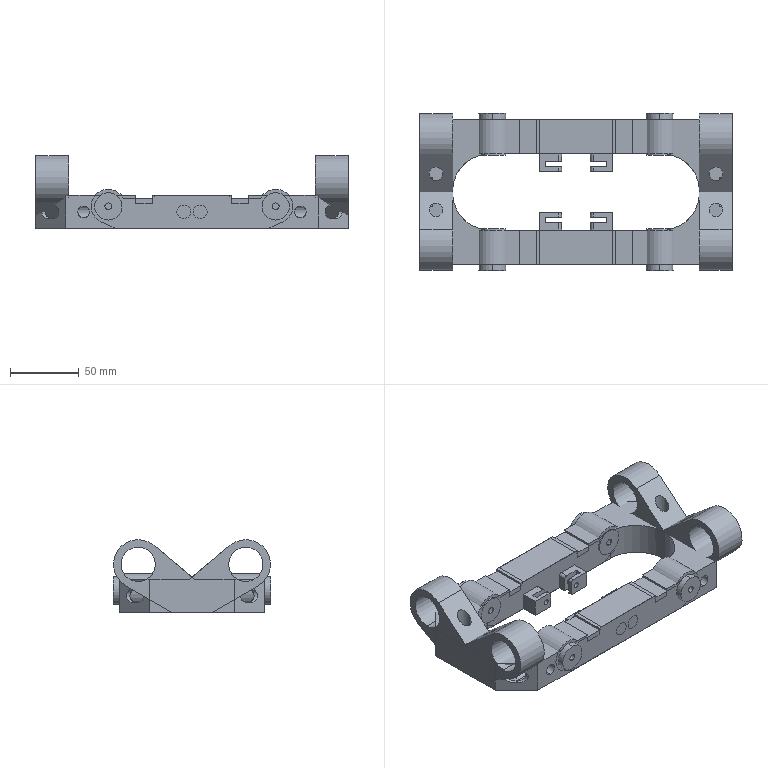NC program | Mastercam | posted with a generic post | part box 228 x 114.503 x 53 mm
Lines 1 to 872 of 11407:
%
:0001()
(MATERIAL - ALUMINUM MM - 2024)
(T12|12 FEM |H12|XY STOCK TO LEAVE - .25|Z STOCK TO LEAVE - .2)
(T7|6 CHM |H7)
(T3|10 BM/BNOS |H3)
(T4|4 BM/BNOS |H4)
N100 G21
N102 G0 G17 G40 G80 G90 G94 G98
N104 G0 G28 G91 Z0.
N106 G0 G28 X0. Y0.
(12 FEM |TOOL - 12|DIA. OFF. - 12|LEN. - 12|TOOL DIA. - 12.)
N108 T12 M6
N110 G0 G54 G90 X181.749 Y4.475 C0. B0. S6000 M3
N112 G43 H12 Z118.
N114 Z41.
N116 G1 Z38.275 F600.
N118 Y5.677 Z38.239 F6000.
N120 G3 X178.852 Y8.574 Z38.134 I-2.897
N122 G1 X177.889 Z38.121
N124 X166.677 Z37.774
N126 G3 X164.717 Y7.973 Z37.712 J-3.498
N128 X163.761 Y7.008 Z37.67 I1.96 J-2.897
N130 G2 X160.254 Y2.986 Z37.508 I-18.624 J12.704
N132 G3 X159.975 Y2.379 I.521 J-.607
N134 X160.775 Y1.578 I.8
N136 G1 X163.085
N138 X178.852
N140 G3 X181.749 Y4.475 J2.897
N142 G1 Y5.677
N144 G3 X178.852 Y8.574 I-2.897
N146 G1 X172.464
N148 X166.677
N150 G3 X163.761 Y7.008 J-3.498
N152 G2 X160.254 Y2.986 I-18.624 J12.704
N154 G3 X159.975 Y2.379 I.521 J-.607
N156 X160.775 Y1.578 I.8
N158 G1 X163.085
N160 G2 X164.255 Y.741 J-1.238
N162 G1 X165.626 Y-3.263
N164 G3 X166.797 Y-4.1 I1.171 J.401
N166 G1 X184.529
N168 G3 X187.427 Y-1.203 J2.897
N170 G1 Y11.354
N172 G3 X184.529 Y14.251 I-2.898
N174 G1 X172.464
N176 X164.58
N178 G3 X159.608 Y11.184 J-5.563
N180 G2 X155.054 Y6.215 I-12.896 J7.248
N182 G3 X153.144 Y2.669 I2.337 J-3.546
N184 X153.183 Y2.093 I4.247
N186 G1 X153.297 Y-1.203
N188 G3 X156.194 Y-4.1 I2.897
N190 G1 X166.797
N192 G0 Z117.508
N194 X95.034 Y-4.711
N196 Z41.
N198 G1 Z38.275 F600.
N200 X100.077 Z38.121 F6000.
N202 X109.514 Z37.829
N204 G3 X112.412 Y-1.823 Z37.718 J2.898
N206 G2 X112.422 Y-1.462 Z37.712 I18.322 J-.319
N208 X113.108 Y2.869 Z37.576 I18.312 J-.68
N210 G3 X113.191 Y3.362 Z37.565 I-1.418 J.493
N212 X111.69 Y4.863 Z37.515 I-1.501
N214 G1 X110.537 Z37.508
N216 X102.317
N218 X95.034
N220 G3 X92.137 Y1.966 J-2.897
N222 G1 Y-1.814
N224 G3 X95.034 Y-4.711 I2.897
N226 G1 X109.514
N228 G3 X112.412 Y-1.823 J2.898
N230 G2 X113.108 Y2.869 I18.322 J-.319
N232 G3 X113.191 Y3.362 I-1.418 J.493
N234 X111.69 Y4.863 I-1.501
N236 G1 X110.537
N238 G2 X109.361 Y5.718 J1.238
N240 G1 X108.002 Y9.895
N242 G3 X106.825 Y10.75 I-1.177 J-.382
N244 G1 X86.541
N246 G3 X86.25 Y10.459 J-.291
N248 G1 Y-10.307
N250 G3 X86.542 Y-10.598 I.292
N252 G1 X118.006
N254 G3 X118.298 Y-10.306 J.292
N256 G1 Y-2.076
N258 G2 X118.287 Y-1.641 I8.592 J.435
N260 X119.754 Y3.163 I8.603
N262 X123.642 Y6.205 I6.736 J-4.603
N264 X126.532 Y6.75 I2.957 J-7.748
N266 G1 X140.088
N268 G2 X140.431 Y6.759 I.343 J-6.558
N270 X143.853 Y5.797 J-6.567
N272 X146.476 Y2.441 I-3.226 J-5.224
N274 G1 X146.679 Y1.688
N276 X146.782 Y.936
N278 X146.798 Y-10.307
N280 G3 X147.09 Y-10.598 I.292
N282 G1 X193.634
N284 G3 X193.925 Y-10.307 J.291
N286 G1 Y20.458
N288 G3 X193.634 Y20.75 I-.291
N290 G1 X154.831
N292 G3 X154.541 Y20.46 J-.29
N294 G1 Y17.497
N296 G2 X154.551 Y17.126 I-6.551 J-.371
N298 X153.076 Y12.98 I-6.561
N300 X149.878 Y10.964 I-4.832 J4.119
N302 G1 X149.125 Y10.808
N304 X148.372 Y10.751
N306 X106.825 Y10.75
N308 G0 Z117.508
N310 X143.374 Y-3.656
N312 Z41.
N314 G1 Z38.125 F600.
N316 G3 X144.93 Y-1.088 Z38.028 I-1.341 J2.568 F6000.
N318 G1 X144.929 Y.087 Z37.994
N320 G3 X143.754 Y2.933 Z37.913 I-4.06 J-.011
N322 X140.869 Y4.136 Z37.812 I-2.885 J-2.857
N324 G1 X137.265 Z37.7
N326 X124.873
N328 G3 X120.212 Y-.942 I.61 J-5.238
N330 X120.204 Y-1.152 I2.825 J-.21
N332 X123.037 Y-3.985 I2.833
N334 G1 X132.871
N336 X142.033
N338 G3 X144.93 Y-1.088 J2.897
N340 G1 X144.929 Y.087
N342 G3 X140.869 Y4.136 I-4.06 J-.011
N344 G1 X137.265
N346 G2 X136.072 Y5.044 J1.238
N348 G1 X134.745 Y9.842
N350 G3 X133.552 Y10.75 I-1.193 J-.33
N352 G1 X119.712
N354 G3 X119.62 Y10.658 J-.092
N356 X119.641 Y10.601 I.092
N358 G1 X119.954 Y10.208
N360 X119.546 Y9.463
N362 G3 X115.765 Y5.739 I7.889 J-11.791
N364 X114.051 Y2.016 I11.253 J-7.438
N366 X113.579 Y-.963 I12.834 J-3.561
N368 G1 X113.553 Y-1.708
N370 X113.552 Y-9.9
N372 X113.481 Y-10.276
N374 G3 X113.476 Y-10.326 I.268 J-.05
N376 X113.749 Y-10.598 I.273
N378 G1 X132.871
N380 X151.456
N382 G3 X151.667 Y-10.387 J.211
N384 X151.66 Y-10.333 I-.211
N386 G1 X151.544 Y-9.9
N388 X151.542 Y.526
N390 G3 X151.109 Y3.505 I-12.006 J-.225
N392 X149.461 Y6.91 I-10.593 J-3.023
N394 G1 X149.236 Y7.229
N396 X148.6 Y7.974
N398 X147.962 Y8.604
N400 X146.984 Y9.463
N402 X146.622 Y10.398
N404 G3 X146.075 Y10.75 I-.547 J-.248
N406 G1 X133.552
N408 G0 Z117.7
N410 X181.684 Y4.54
N412 Z117.508
N414 Z40.508
N416 G1 Z37.767 F600.
N418 Y5.612 Z37.735 F6000.
N420 G3 X178.787 Y8.509 Z37.637 I-2.897
N422 G1 X178.044 Z37.628
N424 X166.675 Z37.276
N426 G3 X164.864 Y7.993 Z37.22 J-3.433
N428 X163.779 Y6.92 Z37.172 I1.811 J-2.917
N430 G2 X160.059 Y2.756 Z37.015 I-19.438 J13.624
N432 G3 X159.83 Y2.271 I.4 J-.485
N434 X160.459 Y1.643 I.629
N436 G1 X163.065
N438 X178.787
N440 G3 X181.684 Y4.54 J2.897
N442 G1 Y5.612
N444 G3 X178.787 Y8.509 I-2.897
N446 G1 X172.463
N448 X166.675
N450 G3 X163.779 Y6.92 J-3.433
N452 G2 X160.059 Y2.756 I-19.438 J13.624
N454 G3 X159.83 Y2.271 I.4 J-.485
N456 X160.459 Y1.643 I.629
N458 G1 X163.065
N460 G2 X164.228 Y.827 J-1.238
N462 G1 X165.614 Y-2.998
N464 G3 X166.777 Y-3.814 I1.163 J.421
N466 G1 X184.244
N468 G3 X187.141 Y-.917 J2.897
N470 G1 Y11.069
N472 G3 X184.244 Y13.966 I-2.897
N474 G1 X172.463
N476 X164.834
N478 G3 X159.81 Y10.928 J-5.673
N480 G2 X154.846 Y5.756 I-13.399 J7.892
N482 G3 X153.144 Y2.915 I1.52 J-2.841
N484 X153.188 Y2.385 I3.222
N486 G1 X153.332 Y-.917
N488 G3 X156.229 Y-3.814 I2.897
N490 G1 X166.777
N492 G0 Z117.015
N494 X95.324 Y-4.422
N496 Z40.508
N498 G1 Z37.761 F600.
N500 X99.741 Z37.628 F6000.
N502 X109.473 Z37.327
N504 G3 X112.366 Y-1.728 Z37.22 J2.9
N506 G1 X112.373 Y-1.581 Z37.215
N508 G2 X112.962 Y2.544 Z37.086 I17.169 J-.348
N510 G3 X113.033 Y3.01 Z37.076 I-1.492 J.466
N512 X111.47 Y4.573 Z37.023 I-1.563
N514 G1 X110.405 Z37.015
N516 X102.437
N518 X95.324
N520 G3 X92.427 Y1.676 J-2.897
N522 G1 Y-1.525
N524 G3 X95.324 Y-4.422 I2.897
N526 G1 X109.473
N528 G3 X112.373 Y-1.581 J2.9
N530 G2 X112.962 Y2.544 I17.169 J-.348
N532 G3 X113.033 Y3.01 I-1.492 J.466
N534 X111.47 Y4.573 I-1.563
N536 G1 X110.405
N538 G2 X109.227 Y5.431 J1.238
N540 G1 X107.87 Y9.642
N542 G3 X106.693 Y10.5 I-1.177 J-.38
N544 G1 X86.791
N546 G3 X86.5 Y10.209 J-.291
N548 G1 Y-10.057
N550 G3 X86.792 Y-10.348 I.292
N552 G1 X118.008
N554 G3 X118.298 Y-10.059 J.289
N556 G1 Y-1.701
N558 G2 X118.296 Y-1.528 I8.276 J.173
N560 X123.892 Y6.303 I8.278
N562 X126.152 Y6.737 I2.823 J-8.61
N564 G1 X126.905 Y6.75
N566 X140.464
N568 X140.468
N570 G2 X144.231 Y5.546 J-6.481
N572 X146.333 Y2.817 I-3.557 J-4.914
N574 X146.798 Y.558 I-5.779 J-2.367
N576 G1 Y-10.057
N578 G3 X147.09 Y-10.348 I.292
N580 G1 X193.384
N582 G3 X193.675 Y-10.057 J.291
N584 G1 Y20.208
N586 G3 X193.384 Y20.5 I-.291
N588 G1 X155.081
N590 G3 X154.791 Y20.21 J-.29
N592 G1 Y17.124
N594 G2 X154.792 Y17.031 I-6.523 J-.093
N596 X150.257 Y10.818 I-6.524
N598 X148.162 Y10.498 I-2.095 J6.699
N600 X147.997 Y10.5 J7.019
N602 G1 X133.685
N604 X106.693
N606 G0 Z117.015
N608 X181.749 Y4.475
N610 Z40.015
N612 G1 Z37.29 F600.
N614 Y5.677 Z37.254 F6000.
N616 G3 X178.852 Y8.574 Z37.15 I-2.897
N618 G1 X177.889 Z37.136
N620 X166.677 Z36.789
N622 G3 X164.717 Y7.973 Z36.727 J-3.498
N624 X163.761 Y7.008 Z36.685 I1.96 J-2.897
N626 G2 X160.254 Y2.986 Z36.523 I-18.624 J12.704
N628 G3 X159.975 Y2.379 I.521 J-.607
N630 X160.775 Y1.578 I.8
N632 G1 X163.085
N634 X178.852
N636 G3 X181.749 Y4.475 J2.897
N638 G1 Y5.677
N640 G3 X178.852 Y8.574 I-2.897
N642 G1 X172.464
N644 X166.677
N646 G3 X163.761 Y7.008 J-3.498
N648 G2 X160.254 Y2.986 I-18.624 J12.704
N650 G3 X159.975 Y2.379 I.521 J-.607
N652 X160.775 Y1.578 I.8
N654 G1 X163.085
N656 G2 X164.255 Y.741 J-1.238
N658 G1 X165.626 Y-3.263
N660 G3 X166.797 Y-4.1 I1.171 J.401
N662 G1 X184.529
N664 G3 X187.427 Y-1.203 J2.897
N666 G1 Y11.354
N668 G3 X184.529 Y14.251 I-2.898
N670 G1 X172.464
N672 X164.58
N674 G3 X159.608 Y11.184 J-5.563
N676 G2 X155.054 Y6.215 I-12.896 J7.248
N678 G3 X153.144 Y2.669 I2.337 J-3.546
N680 X153.183 Y2.093 I4.247
N682 G1 X153.297 Y-1.203
N684 G3 X156.194 Y-4.1 I2.897
N686 G1 X166.797
N688 G0 Z116.523
N690 X95.034 Y-4.711
N692 Z40.015
N694 G1 Z37.291 F600.
N696 X100.077 Z37.136 F6000.
N698 X109.514 Z36.844
N700 G3 X112.412 Y-1.823 Z36.733 J2.898
N702 G2 X112.422 Y-1.462 Z36.727 I18.322 J-.319
N704 X113.108 Y2.869 Z36.592 I18.312 J-.68
N706 G3 X113.191 Y3.362 Z36.581 I-1.418 J.493
N708 X111.69 Y4.863 Z36.53 I-1.501
N710 G1 X110.537 Z36.523
N712 X102.317
N714 X95.034
N716 G3 X92.137 Y1.966 J-2.897
N718 G1 Y-1.814
N720 G3 X95.034 Y-4.711 I2.897
N722 G1 X109.514
N724 G3 X112.412 Y-1.823 J2.898
N726 G2 X113.108 Y2.869 I18.322 J-.319
N728 G3 X113.191 Y3.362 I-1.418 J.493
N730 X111.69 Y4.863 I-1.501
N732 G1 X110.537
N734 G2 X109.361 Y5.718 J1.238
N736 G1 X108.002 Y9.895
N738 G3 X106.825 Y10.75 I-1.177 J-.382
N740 G1 X86.541
N742 G3 X86.25 Y10.459 J-.291
N744 G1 Y-10.307
N746 G3 X86.542 Y-10.598 I.292
N748 G1 X118.006
N750 G3 X118.298 Y-10.306 J.292
N752 G1 Y-2.076
N754 G2 X118.287 Y-1.641 I8.592 J.435
N756 X119.754 Y3.163 I8.603
N758 X123.642 Y6.205 I6.736 J-4.603
N760 X126.532 Y6.75 I2.957 J-7.748
N762 G1 X140.088
N764 G2 X140.431 Y6.759 I.343 J-6.558
N766 X143.853 Y5.797 J-6.567
N768 X146.476 Y2.441 I-3.226 J-5.224
N770 G1 X146.679 Y1.688
N772 X146.782 Y.936
N774 X146.798 Y-10.307
N776 G3 X147.09 Y-10.598 I.292
N778 G1 X193.634
N780 G3 X193.925 Y-10.307 J.291
N782 G1 Y20.458
N784 G3 X193.634 Y20.75 I-.291
N786 G1 X154.831
N788 G3 X154.541 Y20.46 J-.29
N790 G1 Y17.497
N792 G2 X154.551 Y17.126 I-6.551 J-.371
N794 X153.076 Y12.98 I-6.561
N796 X149.878 Y10.964 I-4.832 J4.119
N798 G1 X149.125 Y10.808
N800 X148.372 Y10.751
N802 X106.825 Y10.75
N804 G0 Z116.523
N806 X181.749 Y4.475
N808 Z39.523
N810 G1 Z36.798 F600.
N812 Y5.677 Z36.762 F6000.
N814 G3 X178.852 Y8.574 Z36.657 I-2.897
N816 G1 X177.889 Z36.644
N818 X166.677 Z36.297
N820 G3 X164.717 Y7.973 Z36.235 J-3.498
N822 X163.761 Y7.008 Z36.193 I1.96 J-2.897
N824 G2 X160.254 Y2.986 Z36.031 I-18.624 J12.704
N826 G3 X159.975 Y2.379 I.521 J-.607
N828 X160.775 Y1.578 I.8
N830 G1 X163.085
N832 X178.852
N834 G3 X181.749 Y4.475 J2.897
N836 G1 Y5.677
N838 G3 X178.852 Y8.574 I-2.897
N840 G1 X172.464
N842 X166.677
N844 G3 X163.761 Y7.008 J-3.498
N846 G2 X160.254 Y2.986 I-18.624 J12.704
N848 G3 X159.975 Y2.379 I.521 J-.607
N850 X160.775 Y1.578 I.8
N852 G1 X163.085
N854 G2 X164.255 Y.741 J-1.238
N856 G1 X165.626 Y-3.263
N858 G3 X166.797 Y-4.1 I1.171 J.401
N860 G1 X184.529
N862 G3 X187.427 Y-1.203 J2.897
N864 G1 Y11.354
N866 G3 X184.529 Y14.251 I-2.898
N868 G1 X172.464
N870 X164.58
N872 G3 X159.608 Y11.184 J-5.563
N874 G2 X155.054 Y6.215 I-12.896 J7.248
N876 G3 X153.144 Y2.669 I2.337 J-3.546
N878 X153.183 Y2.093 I4.247
N880 G1 X153.297 Y-1.203
N882 G3 X156.194 Y-4.1 I2.897
N884 G1 X166.797
N886 G0 Z116.031
N888 X95.034 Y-4.711
N890 Z39.523
N892 G1 Z36.798 F600.
N894 X100.077 Z36.644 F6000.
N896 X109.514 Z36.352
N898 G3 X112.412 Y-1.823 Z36.241 J2.898
N900 G2 X112.422 Y-1.462 Z36.235 I18.322 J-.319
N902 X113.108 Y2.869 Z36.099 I18.312 J-.68
N904 G3 X113.191 Y3.362 Z36.088 I-1.418 J.493
N906 X111.69 Y4.863 Z36.038 I-1.501
N908 G1 X110.537 Z36.031
N910 X102.317
N912 X95.034
N914 G3 X92.137 Y1.966 J-2.897
N916 G1 Y-1.814
N918 G3 X95.034 Y-4.711 I2.897
N920 G1 X109.514
N922 G3 X112.412 Y-1.823 J2.898
N924 G2 X113.108 Y2.869 I18.322 J-.319
N926 G3 X113.191 Y3.362 I-1.418 J.493
N928 X111.69 Y4.863 I-1.501
N930 G1 X110.537
N932 G2 X109.361 Y5.718 J1.238
N934 G1 X108.002 Y9.895
N936 G3 X106.825 Y10.75 I-1.177 J-.382
N938 G1 X86.541
N940 G3 X86.25 Y10.459 J-.291
N942 G1 Y-10.307
N944 G3 X86.542 Y-10.598 I.292
N946 G1 X118.006
N948 G3 X118.298 Y-10.306 J.292
N950 G1 Y-2.076
N952 G2 X118.287 Y-1.641 I8.592 J.435
N954 X119.754 Y3.163 I8.603
N956 X123.642 Y6.205 I6.736 J-4.603
N958 X126.532 Y6.75 I2.957 J-7.748
N960 G1 X140.088
N962 G2 X140.431 Y6.759 I.343 J-6.558
N964 X143.853 Y5.797 J-6.567
N966 X146.476 Y2.441 I-3.226 J-5.224
N968 G1 X146.679 Y1.688
N970 X146.782 Y.936
N972 X146.798 Y-10.307
N974 G3 X147.09 Y-10.598 I.292
N976 G1 X193.634
N978 G3 X193.925 Y-10.307 J.291
N980 G1 Y20.458
N982 G3 X193.634 Y20.75 I-.291
N984 G1 X154.831
N986 G3 X154.541 Y20.46 J-.29
N988 G1 Y17.497
N990 G2 X154.551 Y17.126 I-6.551 J-.371
N992 X153.076 Y12.98 I-6.561
N994 X149.878 Y10.964 I-4.832 J4.119
N996 G1 X149.125 Y10.808
N998 X148.372 Y10.751
N1000 X106.825 Y10.75
N1002 G0 Z116.031
N1004 X181.749 Y4.475
N1006 Z39.031
N1008 G1 Z36.306 F600.
N1010 Y5.677 Z36.269 F6000.
N1012 G3 X178.852 Y8.574 Z36.165 I-2.897
N1014 G1 X177.889 Z36.151
N1016 X166.677 Z35.804
N1018 G3 X164.717 Y7.973 Z35.743 J-3.498
N1020 X163.761 Y7.008 Z35.701 I1.96 J-2.897
N1022 G2 X160.254 Y2.986 Z35.538 I-18.624 J12.704
N1024 G3 X159.975 Y2.379 I.521 J-.607
N1026 X160.775 Y1.578 I.8
N1028 G1 X163.085
N1030 X178.852
N1032 G3 X181.749 Y4.475 J2.897
N1034 G1 Y5.677
N1036 G3 X178.852 Y8.574 I-2.897
N1038 G1 X172.464
N1040 X166.677
N1042 G3 X163.761 Y7.008 J-3.498
N1044 G2 X160.254 Y2.986 I-18.624 J12.704
N1046 G3 X159.975 Y2.379 I.521 J-.607
N1048 X160.775 Y1.578 I.8
N1050 G1 X163.085
N1052 G2 X164.255 Y.741 J-1.238
N1054 G1 X165.626 Y-3.263
N1056 G3 X166.797 Y-4.1 I1.171 J.401
N1058 G1 X184.529
N1060 G3 X187.427 Y-1.203 J2.897
N1062 G1 Y11.354
N1064 G3 X184.529 Y14.251 I-2.898
N1066 G1 X172.464
N1068 X164.58
N1070 G3 X159.608 Y11.184 J-5.563
N1072 G2 X155.054 Y6.215 I-12.896 J7.248
N1074 G3 X153.144 Y2.669 I2.337 J-3.546
N1076 X153.183 Y2.093 I4.247
N1078 G1 X153.297 Y-1.203
N1080 G3 X156.194 Y-4.1 I2.897
N1082 G1 X166.797
N1084 G0 Z115.538
N1086 X95.034 Y-4.711
N1088 Z39.031
N1090 G1 Z36.306 F600.
N1092 X100.077 Z36.151 F6000.
N1094 X109.514 Z35.859
N1096 G3 X112.412 Y-1.823 Z35.748 J2.898
N1098 G2 X112.422 Y-1.462 Z35.743 I18.322 J-.319
N1100 X113.108 Y2.869 Z35.607 I18.312 J-.68
N1102 G3 X113.191 Y3.362 Z35.596 I-1.418 J.493
N1104 X111.69 Y4.863 Z35.546 I-1.501
N1106 G1 X110.537 Z35.538
N1108 X102.317
N1110 X95.034
N1112 G3 X92.137 Y1.966 J-2.897
N1114 G1 Y-1.814
N1116 G3 X95.034 Y-4.711 I2.897
N1118 G1 X109.514
N1120 G3 X112.412 Y-1.823 J2.898
N1122 G2 X113.108 Y2.869 I18.322 J-.319
N1124 G3 X113.191 Y3.362 I-1.418 J.493
N1126 X111.69 Y4.863 I-1.501
N1128 G1 X110.537
N1130 G2 X109.361 Y5.718 J1.238
N1132 G1 X108.002 Y9.895
N1134 G3 X106.825 Y10.75 I-1.177 J-.382
N1136 G1 X86.541
N1138 G3 X86.25 Y10.459 J-.291
N1140 G1 Y-10.307
N1142 G3 X86.542 Y-10.598 I.292
N1144 G1 X118.006
N1146 G3 X118.298 Y-10.306 J.292
N1148 G1 Y-2.076
N1150 G2 X118.287 Y-1.641 I8.592 J.435
N1152 X119.754 Y3.163 I8.603
N1154 X123.642 Y6.205 I6.736 J-4.603
N1156 X126.532 Y6.75 I2.957 J-7.748
N1158 G1 X140.088
N1160 G2 X140.431 Y6.759 I.343 J-6.558
N1162 X143.853 Y5.797 J-6.567
N1164 X146.476 Y2.441 I-3.226 J-5.224
N1166 G1 X146.679 Y1.688
N1168 X146.782 Y.936
N1170 X146.798 Y-10.307
N1172 G3 X147.09 Y-10.598 I.292
N1174 G1 X193.634
N1176 G3 X193.925 Y-10.307 J.291
N1178 G1 Y20.458
N1180 G3 X193.634 Y20.75 I-.291
N1182 G1 X154.831
N1184 G3 X154.541 Y20.46 J-.29
N1186 G1 Y17.497
N1188 G2 X154.551 Y17.126 I-6.551 J-.371
N1190 X153.076 Y12.98 I-6.561
N1192 X149.878 Y10.964 I-4.832 J4.119
N1194 G1 X149.125 Y10.808
N1196 X148.372 Y10.751
N1198 X106.825 Y10.75
N1200 G0 Z115.538
N1202 X181.749 Y4.475
N1204 Z38.538
N1206 G1 Z35.813 F600.
N1208 Y5.677 Z35.777 F6000.
N1210 G3 X178.852 Y8.574 Z35.673 I-2.897
N1212 G1 X177.889 Z35.659
N1214 X166.677 Z35.312
N1216 G3 X164.717 Y7.973 Z35.25 J-3.498
N1218 X163.761 Y7.008 Z35.208 I1.96 J-2.897
N1220 G2 X160.254 Y2.986 Z35.046 I-18.624 J12.704
N1222 G3 X159.975 Y2.379 I.521 J-.607
N1224 X160.775 Y1.578 I.8
N1226 G1 X163.085
N1228 X178.852
N1230 G3 X181.749 Y4.475 J2.897
N1232 G1 Y5.677
N1234 G3 X178.852 Y8.574 I-2.897
N1236 G1 X172.464
N1238 X166.677
N1240 G3 X163.761 Y7.008 J-3.498
N1242 G2 X160.254 Y2.986 I-18.624 J12.704
N1244 G3 X159.975 Y2.379 I.521 J-.607
N1246 X160.775 Y1.578 I.8
N1248 G1 X163.085
N1250 G2 X164.255 Y.741 J-1.238
N1252 G1 X165.626 Y-3.263
N1254 G3 X166.797 Y-4.1 I1.171 J.401
N1256 G1 X184.529
N1258 G3 X187.427 Y-1.203 J2.897
N1260 G1 Y11.354
N1262 G3 X184.529 Y14.251 I-2.898
N1264 G1 X172.464
N1266 X164.58
N1268 G3 X159.608 Y11.184 J-5.563
N1270 G2 X155.054 Y6.215 I-12.896 J7.248
N1272 G3 X153.144 Y2.669 I2.337 J-3.546
N1274 X153.183 Y2.093 I4.247
N1276 G1 X153.297 Y-1.203
N1278 G3 X156.194 Y-4.1 I2.897
N1280 G1 X166.797
N1282 G0 Z115.046
N1284 X95.034 Y-4.711
N1286 Z38.538
N1288 G1 Z35.814 F600.
N1290 X100.077 Z35.659 F6000.
N1292 X109.514 Z35.367
N1294 G3 X112.412 Y-1.823 Z35.256 J2.898
N1296 G2 X112.422 Y-1.462 Z35.25 I18.322 J-.319
N1298 X113.108 Y2.869 Z35.115 I18.312 J-.68
N1300 G3 X113.191 Y3.362 Z35.104 I-1.418 J.493
N1302 X111.69 Y4.863 Z35.053 I-1.501
N1304 G1 X110.537 Z35.046
N1306 X102.317
N1308 X95.034
N1310 G3 X92.137 Y1.966 J-2.897
N1312 G1 Y-1.814
N1314 G3 X95.034 Y-4.711 I2.897
N1316 G1 X109.514
N1318 G3 X112.412 Y-1.823 J2.898
N1320 G2 X113.108 Y2.869 I18.322 J-.319
N1322 G3 X113.191 Y3.362 I-1.418 J.493
N1324 X111.69 Y4.863 I-1.501
N1326 G1 X110.537
N1328 G2 X109.361 Y5.718 J1.238
N1330 G1 X108.002 Y9.895
N1332 G3 X106.825 Y10.75 I-1.177 J-.382
N1334 G1 X86.541
N1336 G3 X86.25 Y10.459 J-.291
N1338 G1 Y-10.307
N1340 G3 X86.542 Y-10.598 I.292
N1342 G1 X118.006
N1344 G3 X118.298 Y-10.306 J.292
N1346 G1 Y-2.076
N1348 G2 X118.287 Y-1.641 I8.592 J.435
N1350 X119.754 Y3.163 I8.603
N1352 X123.642 Y6.205 I6.736 J-4.603
N1354 X126.532 Y6.75 I2.957 J-7.748
N1356 G1 X140.088
N1358 G2 X140.431 Y6.759 I.343 J-6.558
N1360 X143.853 Y5.797 J-6.567
N1362 X146.476 Y2.441 I-3.226 J-5.224
N1364 G1 X146.679 Y1.688
N1366 X146.782 Y.936
N1368 X146.798 Y-10.307
N1370 G3 X147.09 Y-10.598 I.292
N1372 G1 X193.634
N1374 G3 X193.925 Y-10.307 J.291
N1376 G1 Y20.458
N1378 G3 X193.634 Y20.75 I-.291
N1380 G1 X154.831
N1382 G3 X154.541 Y20.46 J-.29
N1384 G1 Y17.497
N1386 G2 X154.551 Y17.126 I-6.551 J-.371
N1388 X153.076 Y12.98 I-6.561
N1390 X149.878 Y10.964 I-4.832 J4.119
N1392 G1 X149.125 Y10.808
N1394 X148.372 Y10.751
N1396 X106.825 Y10.75
N1398 G0 Z115.046
N1400 X181.749 Y4.475
N1402 Z38.046
N1404 G1 Z35.321 F600.
N1406 Y5.677 Z35.285 F6000.
N1408 G3 X178.852 Y8.574 Z35.181 I-2.897
N1410 G1 X177.889 Z35.167
N1412 X166.677 Z34.82
N1414 G3 X164.717 Y7.973 Z34.758 J-3.498
N1416 X163.761 Y7.008 Z34.716 I1.96 J-2.897
N1418 G2 X160.254 Y2.986 Z34.554 I-18.624 J12.704
N1420 G3 X159.975 Y2.379 I.521 J-.607
N1422 X160.775 Y1.578 I.8
N1424 G1 X163.085
N1426 X178.852
N1428 G3 X181.749 Y4.475 J2.897
N1430 G1 Y5.677
N1432 G3 X178.852 Y8.574 I-2.897
N1434 G1 X172.464
N1436 X166.677
N1438 G3 X163.761 Y7.008 J-3.498
N1440 G2 X160.254 Y2.986 I-18.624 J12.704
N1442 G3 X159.975 Y2.379 I.521 J-.607
N1444 X160.775 Y1.578 I.8
N1446 G1 X163.085
N1448 G2 X164.255 Y.741 J-1.238
N1450 G1 X165.626 Y-3.263
N1452 G3 X166.797 Y-4.1 I1.171 J.401
N1454 G1 X184.529
N1456 G3 X187.427 Y-1.203 J2.897
N1458 G1 Y11.354
N1460 G3 X184.529 Y14.251 I-2.898
N1462 G1 X172.464
N1464 X164.58
N1466 G3 X159.608 Y11.184 J-5.563
N1468 G2 X155.054 Y6.215 I-12.896 J7.248
N1470 G3 X153.144 Y2.669 I2.337 J-3.546
N1472 X153.183 Y2.093 I4.247
N1474 G1 X153.297 Y-1.203
N1476 G3 X156.194 Y-4.1 I2.897
N1478 G1 X166.797
N1480 G0 Z114.554
N1482 X95.034 Y-4.711
N1484 Z38.046
N1486 G1 Z35.321 F600.
N1488 X100.077 Z35.167 F6000.
N1490 X109.514 Z34.875
N1492 G3 X112.412 Y-1.823 Z34.764 J2.898
N1494 G2 X112.422 Y-1.462 Z34.758 I18.322 J-.319
N1496 X113.108 Y2.869 Z34.622 I18.312 J-.68
N1498 G3 X113.191 Y3.362 Z34.611 I-1.418 J.493
N1500 X111.69 Y4.863 Z34.561 I-1.501
N1502 G1 X110.537 Z34.554
N1504 X102.317
N1506 X95.034
N1508 G3 X92.137 Y1.966 J-2.897
N1510 G1 Y-1.814
N1512 G3 X95.034 Y-4.711 I2.897
N1514 G1 X109.514
N1516 G3 X112.412 Y-1.823 J2.898
N1518 G2 X113.108 Y2.869 I18.322 J-.319
N1520 G3 X113.191 Y3.362 I-1.418 J.493
N1522 X111.69 Y4.863 I-1.501
N1524 G1 X110.537
N1526 G2 X109.361 Y5.718 J1.238
N1528 G1 X108.002 Y9.895
N1530 G3 X106.825 Y10.75 I-1.177 J-.382
N1532 G1 X86.541
N1534 G3 X86.25 Y10.459 J-.291
N1536 G1 Y-10.307
N1538 G3 X86.542 Y-10.598 I.292
N1540 G1 X118.006
N1542 G3 X118.298 Y-10.306 J.292
N1544 G1 Y-2.076
N1546 G2 X118.287 Y-1.641 I8.592 J.435
N1548 X119.754 Y3.163 I8.603
N1550 X123.642 Y6.205 I6.736 J-4.603
N1552 X126.532 Y6.75 I2.957 J-7.748
N1554 G1 X140.088
N1556 G2 X140.431 Y6.759 I.343 J-6.558
N1558 X143.853 Y5.797 J-6.567
N1560 X146.476 Y2.441 I-3.226 J-5.224
N1562 G1 X146.679 Y1.688
N1564 X146.782 Y.936
N1566 X146.798 Y-10.307
N1568 G3 X147.09 Y-10.598 I.292
N1570 G1 X193.634
N1572 G3 X193.925 Y-10.307 J.291
N1574 G1 Y20.458
N1576 G3 X193.634 Y20.75 I-.291
N1578 G1 X154.831
N1580 G3 X154.541 Y20.46 J-.29
N1582 G1 Y17.497
N1584 G2 X154.551 Y17.126 I-6.551 J-.371
N1586 X153.076 Y12.98 I-6.561
N1588 X149.878 Y10.964 I-4.832 J4.119
N1590 G1 X149.125 Y10.808
N1592 X148.372 Y10.751
N1594 X106.825 Y10.75
N1596 G0 Z114.554
N1598 X181.749 Y4.475
N1600 Z37.554
N1602 G1 Z34.829 F600.
N1604 Y5.677 Z34.792 F6000.
N1606 G3 X178.852 Y8.574 Z34.688 I-2.897
N1608 G1 X177.889 Z34.675
N1610 X166.677 Z34.327
N1612 G3 X164.717 Y7.973 Z34.266 J-3.498
N1614 X163.761 Y7.008 Z34.224 I1.96 J-2.897
N1616 G2 X160.254 Y2.986 Z34.062 I-18.624 J12.704
N1618 G3 X159.975 Y2.379 I.521 J-.607
N1620 X160.775 Y1.578 I.8
N1622 G1 X163.085
N1624 X178.852
N1626 G3 X181.749 Y4.475 J2.897
N1628 G1 Y5.677
N1630 G3 X178.852 Y8.574 I-2.897
N1632 G1 X172.464
N1634 X166.677
N1636 G3 X163.761 Y7.008 J-3.498
N1638 G2 X160.254 Y2.986 I-18.624 J12.704
N1640 G3 X159.975 Y2.379 I.521 J-.607
N1642 X160.775 Y1.578 I.8
N1644 G1 X163.085
N1646 G2 X164.255 Y.741 J-1.238
N1648 G1 X165.626 Y-3.263
N1650 G3 X166.797 Y-4.1 I1.171 J.401
N1652 G1 X184.529
N1654 G3 X187.427 Y-1.203 J2.897
N1656 G1 Y11.354
N1658 G3 X184.529 Y14.251 I-2.898
N1660 G1 X172.464
N1662 X164.58
N1664 G3 X159.608 Y11.184 J-5.563
N1666 G2 X155.054 Y6.215 I-12.896 J7.248
N1668 G3 X153.144 Y2.669 I2.337 J-3.546
N1670 X153.183 Y2.093 I4.247
N1672 G1 X153.297 Y-1.203
N1674 G3 X156.194 Y-4.1 I2.897
N1676 G1 X166.797
N1678 G0 Z114.062
N1680 X95.034 Y-4.711
N1682 Z37.554
N1684 G1 Z34.829 F600.
N1686 X100.077 Z34.675 F6000.
N1688 X109.514 Z34.382
N1690 G3 X112.412 Y-1.823 Z34.271 J2.898
N1692 G2 X112.422 Y-1.462 Z34.266 I18.322 J-.319
N1694 X113.108 Y2.869 Z34.13 I18.312 J-.68
N1696 G3 X113.191 Y3.362 Z34.119 I-1.418 J.493
N1698 X111.69 Y4.863 Z34.069 I-1.501
N1700 G1 X110.537 Z34.062
N1702 X102.317
N1704 X95.034
N1706 G3 X92.137 Y1.966 J-2.897
N1708 G1 Y-1.814
N1710 G3 X95.034 Y-4.711 I2.897
N1712 G1 X109.514
N1714 G3 X112.412 Y-1.823 J2.898
N1716 G2 X113.108 Y2.869 I18.322 J-.319
N1718 G3 X113.191 Y3.362 I-1.418 J.493
N1720 X111.69 Y4.863 I-1.501
N1722 G1 X110.537
N1724 G2 X109.361 Y5.718 J1.238
N1726 G1 X108.002 Y9.895
N1728 G3 X106.825 Y10.75 I-1.177 J-.382
N1730 G1 X86.541
N1732 G3 X86.25 Y10.459 J-.291
N1734 G1 Y-10.307
N1736 G3 X86.542 Y-10.598 I.292
N1738 G1 X118.006
N1740 G3 X118.298 Y-10.306 J.292
N1742 G1 Y-2.076
N1744 G2 X118.287 Y-1.641 I8.592 J.435
N1746 X119.754 Y3.163 I8.603
N1748 X123.642 Y6.205 I6.736 J-4.603
N1750 X126.532 Y6.75 I2.957 J-7.748
N1752 G1 X140.088
N1754 G2 X140.431 Y6.759 I.343 J-6.558
N1756 X143.853 Y5.797 J-6.567
N1758 X146.476 Y2.441 I-3.226 J-5.224
N1760 G1 X146.679 Y1.688
N1762 X146.782 Y.936
N1764 X146.798 Y-10.307
N1766 G3 X147.09 Y-10.598 I.292
N1768 G1 X193.634
N1770 G3 X193.925 Y-10.307 J.291
N1772 G1 Y20.458
N1774 G3 X193.634 Y20.75 I-.291
N1776 G1 X154.831
N1778 G3 X154.541 Y20.46 J-.29
N1780 G1 Y17.497
N1782 G2 X154.551 Y17.126 I-6.551 J-.371
N1784 X153.076 Y12.98 I-6.561
N1786 X149.878 Y10.964 I-4.832 J4.119
N1788 G1 X149.125 Y10.808
N1790 X148.372 Y10.751
N1792 X106.825 Y10.75
N1794 G0 Z114.062
N1796 X181.749 Y4.475
N1798 Z37.062
N1800 G1 Z34.336 F600.
N1802 Y5.677 Z34.3 F6000.
N1804 G3 X178.852 Y8.574 Z34.196 I-2.897
N1806 G1 X177.889 Z34.182
N1808 X166.677 Z33.835
N1810 G3 X164.717 Y7.973 Z33.774 J-3.498
N1812 X163.761 Y7.008 Z33.732 I1.96 J-2.897
N1814 G2 X160.254 Y2.986 Z33.569 I-18.624 J12.704
N1816 G3 X159.975 Y2.379 I.521 J-.607
N1818 X160.775 Y1.578 I.8
N1820 G1 X163.085
N1822 X178.852
N1824 G3 X181.749 Y4.475 J2.897
N1826 G1 Y5.677